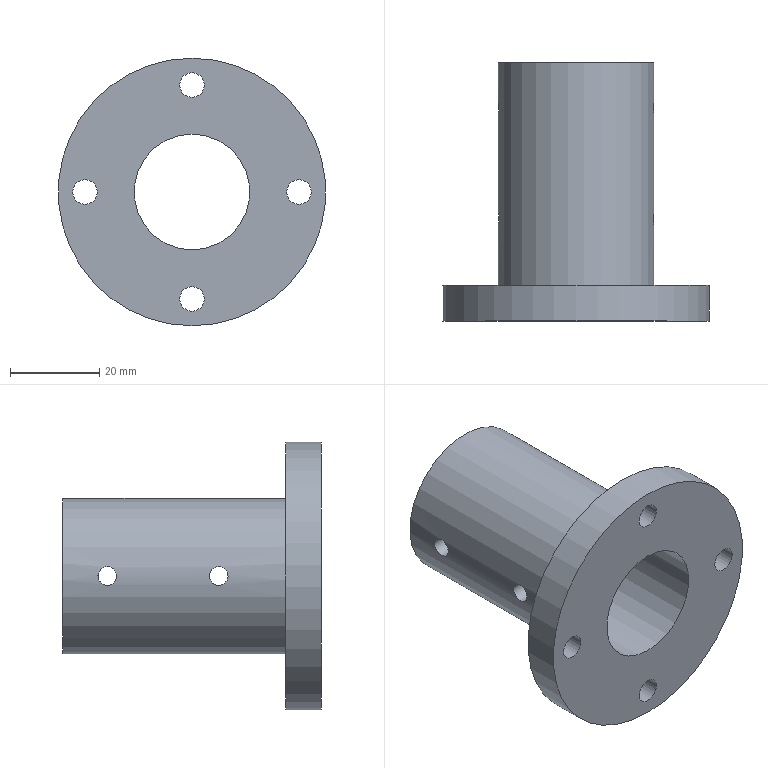Part | STEP file | 1 solid | 14 faces | box 60 x 58 x 60 mm | volume 38921 mm3 | cylinder 11 | plane 3 | commonest cylinder face diameters 4.2 x4 5.5 x4 26 x1 35 x1 60 x1